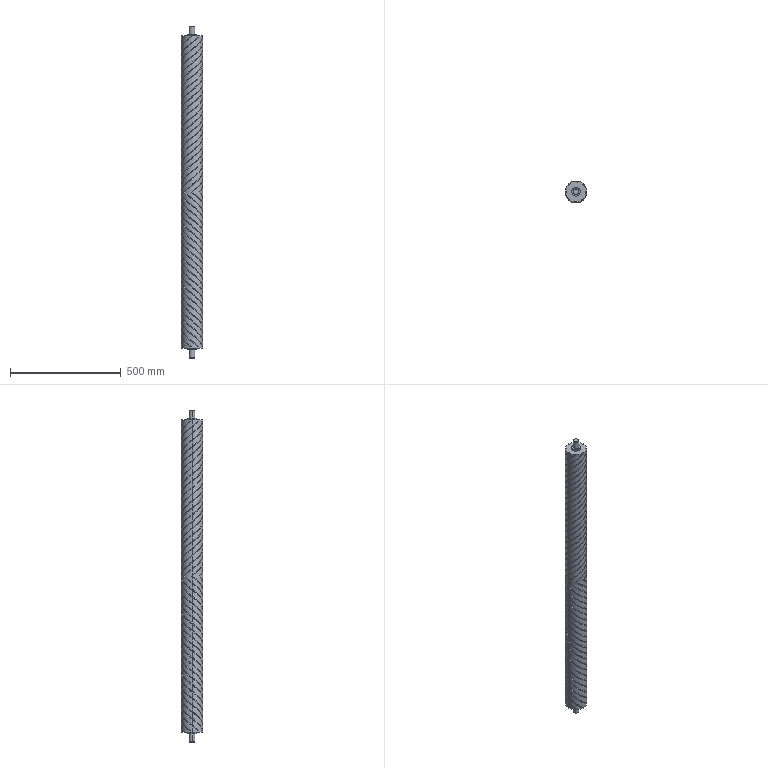Part | SolidWorks | features ICE 4, Helix 2, Chamfer 1, CirPattern 1, Extrusion 1, MirrorPattern 1, SweepCut 1 | 1 solid | 170 faces | box 96 x 96 x 1500 mm | volume 10059847 mm3 | cylinder 108 | spline 48 | cone 8 | plane 6 | commonest cylinder face diameters 96 x100 25 x4 40 x4